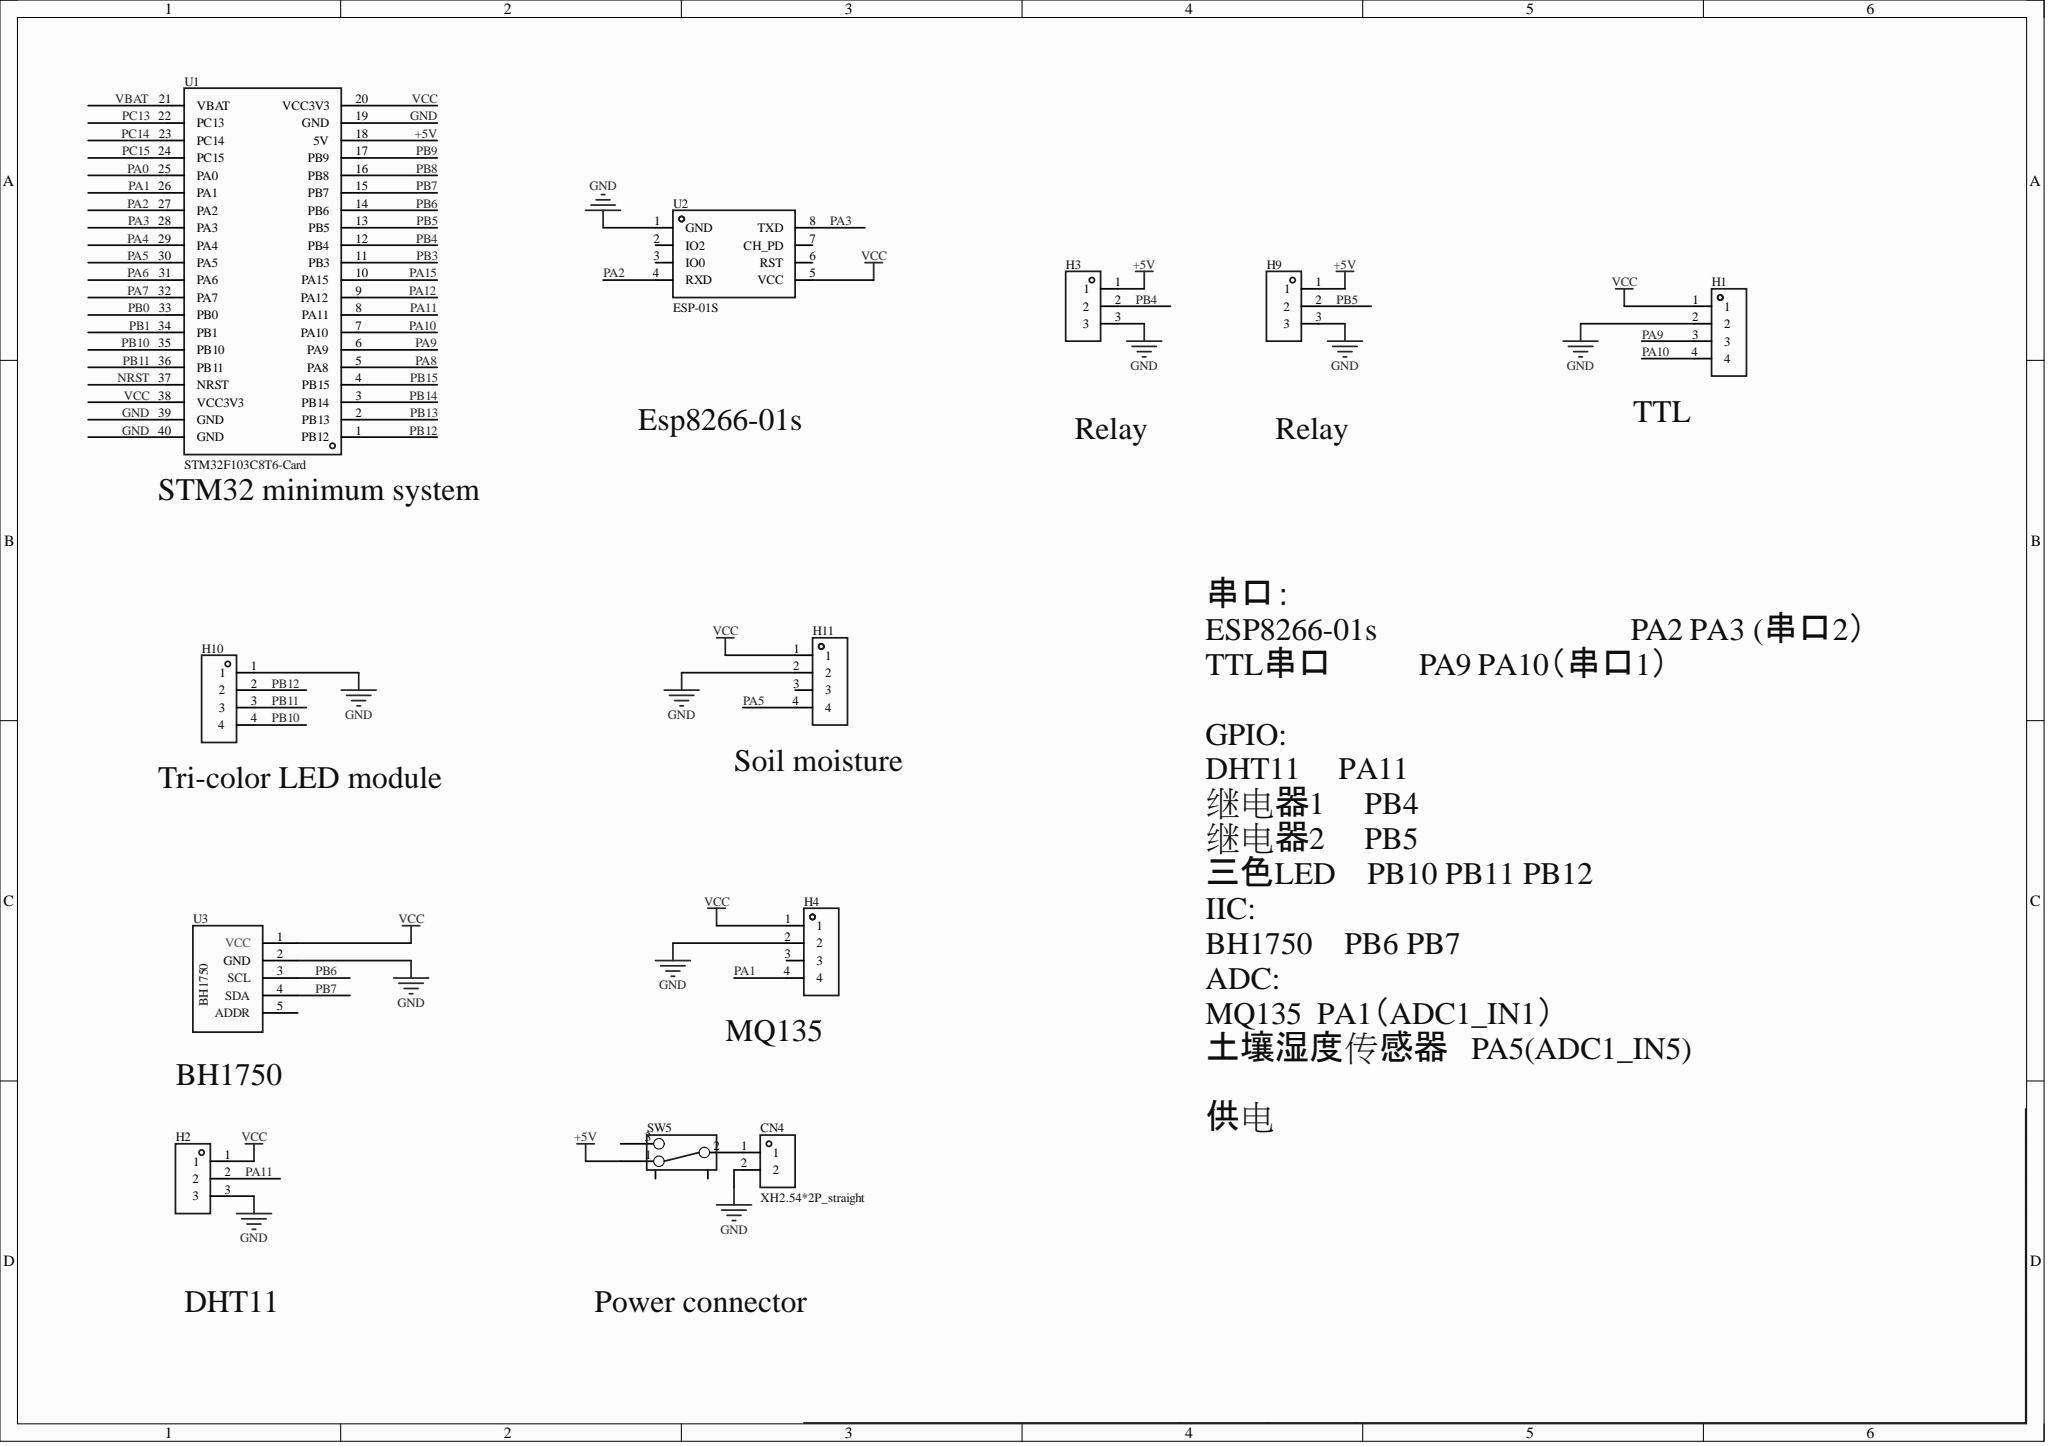Circuit board | Altium Designer | 12 parts | 18 nets
Bill of materials:
Comment,Description,Designator,Footprint,LibRef,Quantity
"XH2.54*2P_straight","","CN4","CONN-TH_2P-P2.50-XH2.54-2P","XH2.54*2P_直插","1"
"","","H1, H4, H10, H11","HDR-TH_4P-P2.54-V-F","HDR-F_2.54_1x4P","4"
"","","H2, H3, H9","HDR-TH_3P-P2.54-V-F","HDR-F_2.54_1x3P","3"
"","","SW5","拨动开关","拨动开关_正","1"
"STM32F103C8T6-Card","","U1","CONN-TH_L53.3-W22.9_STM32F103C8T6-CARD","STM32F103C8T6-Card","1"
"ESP-01S","","U2","WIFIM-TH_ESP-01S","ESP-01S_C111009","1"
"","","U3","BH1750光照传感器","BH1750光照传感器","1"
Netlist (Protel format):
[
CN4
CONN-TH_2P-P2.50-XH2.54-2P
XH2.54*2P_straight



]
[
H1
HDR-TH_4P-P2.54-V-F




]
[
H2
HDR-TH_3P-P2.54-V-F




]
[
H3
HDR-TH_3P-P2.54-V-F




]
[
H4
HDR-TH_4P-P2.54-V-F




]
[
H9
HDR-TH_3P-P2.54-V-F




]
[
H10
HDR-TH_4P-P2.54-V-F




]
[
H11
HDR-TH_4P-P2.54-V-F




]
[
SW5
拨动开关




]
[
U1
CONN-TH_L53.3-W22.9_STM32F103C8T6-CARD
STM32F103C8T6-Card



]
[
U2
WIFIM-TH_ESP-01S
ESP-01S



]
[
U3
BH1750光照传感器




]
(
VCC
H1-1
H2-1
H4-1
H11-1
U1-20
U1-38
U2-5
U3-1
)
(
PB12
H10-2
U1-1
)
(
PB11
H10-3
U1-36
)
(
PB10
H10-4
U1-35
)
(
PB7
U1-15
U3-4
)
(
PB6
U1-14
U3-3
)
(
PB5
H9-2
U1-13
)
(
PB4
H3-2
U1-12
)
(
PA11
H2-2
U1-8
)
(
PA10
H1-4
U1-7
)
(
PA9
H1-3
U1-6
)
(
PA5
H11-4
U1-30
)
(
PA3
U1-28
U2-8
)
(
PA2
U1-27
U2-4
)
(
PA1
H4-4
U1-26
)
(
NetCN4_1
CN4-1
SW5-2
)
(
GND
CN4-2
H1-2
H2-3
H3-3
H4-2
H9-3
H10-1
H11-2
U1-19
U1-39
U1-40
U2-1
U3-2
)
(
+5V
H3-1
H9-1
SW5-1
U1-18
)